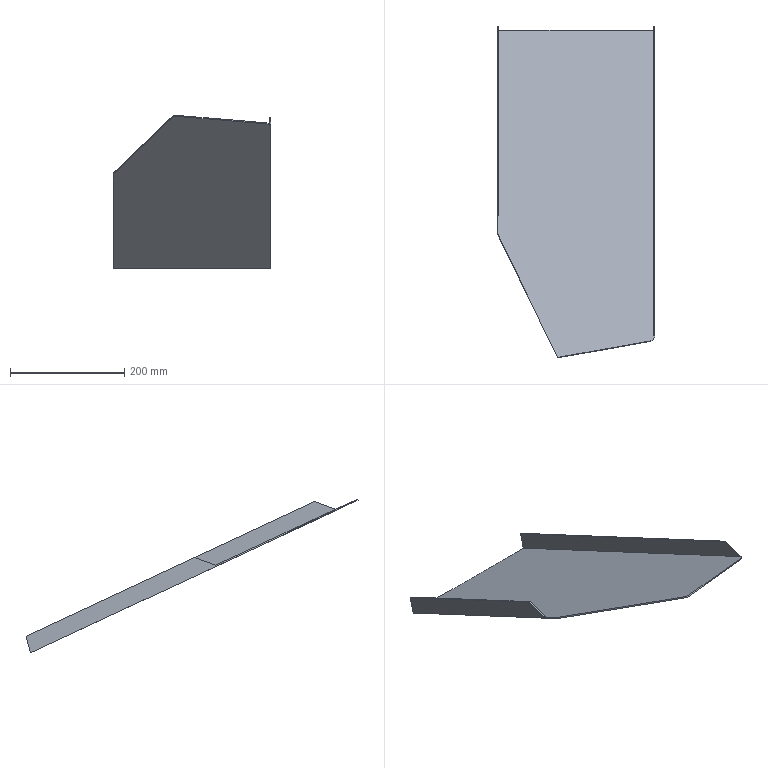Part | NX | features solid 2 | 1 solid | 17 faces | box 276.285 x 582.097 x 269.572 mm | volume 369670 mm3 | plane 16 | spline 1
STEP:
#1=CARTESIAN_POINT('',(829.951,330.323,-255.874));
#2=VERTEX_POINT('',#1);
#3=CARTESIAN_POINT('',(829.951,866.287,-505.798));
#4=VERTEX_POINT('',#3);
#5=CARTESIAN_POINT('',(829.951,540.514,-353.888));
#6=DIRECTION('',(0.,0.9063,-0.4226));
#7=VECTOR('',#6,1000.);
#8=LINE('',#5,#7);
#9=EDGE_CURVE('',#2,#4,#8,.T.);
#10=ORIENTED_EDGE('',*,*,#9,.T.);
#11=CARTESIAN_POINT('',(558.256,866.287,-505.798));
#12=VERTEX_POINT('',#11);
#13=CARTESIAN_POINT('',(831.95,866.287,-505.798));
#14=DIRECTION('',(-1.,0.,0.));
#15=VECTOR('',#14,1000.);
#16=LINE('',#13,#15);
#17=EDGE_CURVE('',#4,#12,#16,.T.);
#18=ORIENTED_EDGE('',*,*,#17,.T.);
#19=CARTESIAN_POINT('',(558.256,540.845,-354.042));
#20=VERTEX_POINT('',#19);
#21=CARTESIAN_POINT('',(558.256,540.514,-353.888));
#22=DIRECTION('',(0.,0.9063,-0.4226));
#23=VECTOR('',#22,1000.);
#24=LINE('',#21,#23);
#25=EDGE_CURVE('',#20,#12,#24,.T.);
#26=ORIENTED_EDGE('',*,*,#25,.F.);
#27=CARTESIAN_POINT('',(556.256,540.845,-354.042));
#28=VERTEX_POINT('',#27);
#29=CARTESIAN_POINT('',(556.256,540.845,-354.042));
#30=DIRECTION('',(-1.,0.,0.));
#31=VECTOR('',#30,1000.);
#32=LINE('',#29,#31);
#33=EDGE_CURVE('',#20,#28,#32,.T.);
#34=ORIENTED_EDGE('',*,*,#33,.T.);
#35=CARTESIAN_POINT('',(555.666,540.845,-354.042));
#36=VERTEX_POINT('',#35);
#37=CARTESIAN_POINT('',(555.666,540.845,-354.042));
#38=DIRECTION('',(1.,0.,0.));
#39=VECTOR('',#38,1000.);
#40=LINE('',#37,#39);
#41=EDGE_CURVE('',#36,#28,#40,.T.);
#42=ORIENTED_EDGE('',*,*,#41,.F.);
#43=CARTESIAN_POINT('',(555.666,510.845,-340.053));
#44=VERTEX_POINT('',#43);
#45=CARTESIAN_POINT('',(555.666,510.845,-340.053));
#46=DIRECTION('',(0.,0.9063,-0.4226));
#47=VECTOR('',#46,1000.);
#48=LINE('',#45,#47);
#49=EDGE_CURVE('',#44,#36,#48,.T.);
#50=ORIENTED_EDGE('',*,*,#49,.F.);
#51=CARTESIAN_POINT('',(556.256,510.845,-340.053));
#52=VERTEX_POINT('',#51);
#53=CARTESIAN_POINT('',(555.666,510.845,-340.053));
#54=DIRECTION('',(1.,0.,0.));
#55=VECTOR('',#54,1000.);
#56=LINE('',#53,#55);
#57=EDGE_CURVE('',#44,#52,#56,.T.);
#58=ORIENTED_EDGE('',*,*,#57,.T.);
#59=CARTESIAN_POINT('',(556.256,509.627,-339.485));
#60=VERTEX_POINT('',#59);
#61=CARTESIAN_POINT('',(556.256,510.845,-340.053));
#62=DIRECTION('',(0.,-0.9063,0.4226));
#63=VECTOR('',#62,1000.);
#64=LINE('',#61,#63);
#65=EDGE_CURVE('',#52,#60,#64,.T.);
#66=ORIENTED_EDGE('',*,*,#65,.T.);
#67=CARTESIAN_POINT('',(661.488,292.393,-238.187));
#68=VERTEX_POINT('',#67);
#69=CARTESIAN_POINT('',(556.256,509.627,-339.485));
#70=DIRECTION('',(0.402,-0.8299,0.387));
#71=VECTOR('',#70,1000.);
#72=LINE('',#69,#71);
#73=EDGE_CURVE('',#60,#68,#72,.T.);
#74=ORIENTED_EDGE('',*,*,#73,.T.);
#75=CARTESIAN_POINT('',(831.951,330.323,-255.874));
#76=VERTEX_POINT('',#75);
#77=CARTESIAN_POINT('',(831.951,330.323,-255.874));
#78=CARTESIAN_POINT('',(831.936,330.109,-255.774));
#79=CARTESIAN_POINT('',(831.91,329.897,-255.675));
#80=CARTESIAN_POINT('',(831.843,329.477,-255.48));
#81=CARTESIAN_POINT('',(831.802,329.269,-255.382));
#82=CARTESIAN_POINT('',(831.703,328.856,-255.19));
#83=CARTESIAN_POINT('',(831.646,328.652,-255.095));
#84=CARTESIAN_POINT('',(831.519,328.246,-254.906));
#85=CARTESIAN_POINT('',(831.448,328.045,-254.812));
#86=CARTESIAN_POINT('',(831.294,327.646,-254.626));
#87=CARTESIAN_POINT('',(831.21,327.448,-254.534));
#88=CARTESIAN_POINT('',(831.074,327.154,-254.396));
#89=CARTESIAN_POINT('',(831.027,327.056,-254.351));
#90=CARTESIAN_POINT('',(830.955,326.91,-254.283));
#91=CARTESIAN_POINT('',(830.93,326.861,-254.26));
#92=CARTESIAN_POINT('',(830.88,326.765,-254.215));
#93=CARTESIAN_POINT('',(830.753,326.524,-254.102));
#94=CARTESIAN_POINT('',(830.619,326.287,-253.992));
#95=CARTESIAN_POINT('',(830.392,325.916,-253.819));
#96=CARTESIAN_POINT('',(830.156,325.55,-253.649));
#97=CARTESIAN_POINT('',(829.771,325.02,-253.401));
#98=CARTESIAN_POINT('',(829.495,324.678,-253.242));
#99=CARTESIAN_POINT('',(829.208,324.342,-253.085));
#100=CARTESIAN_POINT('',(829.06,324.177,-253.008));
#101=CARTESIAN_POINT('',(828.829,323.935,-252.895));
#102=CARTESIAN_POINT('',(828.751,323.855,-252.858));
#103=CARTESIAN_POINT('',(828.592,323.697,-252.784));
#104=CARTESIAN_POINT('',(828.512,323.619,-252.748));
#105=CARTESIAN_POINT('',(828.268,323.389,-252.641));
#106=CARTESIAN_POINT('',(828.101,323.24,-252.572));
#107=CARTESIAN_POINT('',(827.758,322.952,-252.437));
#108=CARTESIAN_POINT('',(827.582,322.813,-252.372));
#109=CARTESIAN_POINT('',(827.222,322.544,-252.247));
#110=CARTESIAN_POINT('',(827.037,322.415,-252.187));
#111=CARTESIAN_POINT('',(826.657,322.167,-252.071));
#112=CARTESIAN_POINT('',(826.462,322.049,-252.016));
#113=CARTESIAN_POINT('',(826.211,321.908,-251.95));
#114=CARTESIAN_POINT('',(826.161,321.881,-251.938));
#115=CARTESIAN_POINT('',(826.059,321.826,-251.912));
#116=CARTESIAN_POINT('',(826.008,321.799,-251.9));
#117=CARTESIAN_POINT('',(825.854,321.72,-251.863));
#118=CARTESIAN_POINT('',(825.75,321.67,-251.839));
#119=CARTESIAN_POINT('',(825.438,321.524,-251.771));
#120=CARTESIAN_POINT('',(825.226,321.435,-251.73));
#121=CARTESIAN_POINT('',(824.797,321.276,-251.655));
#122=CARTESIAN_POINT('',(824.579,321.205,-251.622));
#123=CARTESIAN_POINT('',(824.247,321.113,-251.58));
#124=CARTESIAN_POINT('',(824.135,321.085,-251.567));
#125=CARTESIAN_POINT('',(823.966,321.048,-251.549));
#126=CARTESIAN_POINT('',(823.881,321.03,-251.541));
#127=CARTESIAN_POINT('',(823.795,321.013,-251.533));
#128=CARTESIAN_POINT('',(823.738,321.003,-251.528));
#129=CARTESIAN_POINT('',(823.71,320.998,-251.526));
#130=CARTESIAN_POINT('',(822.765,320.831,-251.448));
#131=CARTESIAN_POINT('',(820.016,320.346,-251.222));
#132=CARTESIAN_POINT('',(809.936,318.569,-250.393));
#133=CARTESIAN_POINT('',(786.111,314.368,-248.434));
#134=CARTESIAN_POINT('',(734.796,305.32,-244.215));
#135=CARTESIAN_POINT('',(690.811,297.564,-240.598));
#136=CARTESIAN_POINT('',(661.488,292.393,-238.187));
#137=B_SPLINE_CURVE_WITH_KNOTS('',3,(#77,#78,#79,#80,#81,#82,#83,#84,#85,#86,#87,#88,#89,#90,#91,#92,#93,#94,#95,#96,#97,#98,#99,#100,#101,#102,#103,#104,#105,#106,#107,#108,#109,#110,#111,#112,#113,#114,#115,#116,#117,#118,#119,#120,#121,#122,#123,#124,#125,#126,#127,#128,#129,#130,#131,#132,#133,#134,#135,#136),.UNSPECIFIED.,.F.,.F.,(4,2,2,2,2,2,2,2,1,2,1,1,2,2,2,2,2,2,2,2,2,2,2,2,2,2,1,2,2,1,1,1,1,4),(0.,0.003906,0.007812,0.01172,0.01562,0.01953,0.02148,0.02246,0.02344,0.02734,0.03125,0.03516,0.03906,0.04297,0.04492,0.04687,0.05078,0.05469,0.05859,0.0625,0.06348,0.06445,0.06641,0.07031,0.07422,0.07617,0.07715,0.07764,0.07812,0.09375,0.125,0.25,0.5,1.),.UNSPECIFIED.);
#138=EDGE_CURVE('',#76,#68,#137,.T.);
#139=ORIENTED_EDGE('',*,*,#138,.F.);
#140=CARTESIAN_POINT('',(831.951,330.323,-255.874));
#141=DIRECTION('',(1.,0.,0.));
#142=VECTOR('',#141,1000.);
#143=LINE('',#140,#142);
#144=EDGE_CURVE('',#76,#2,#143,.F.);
#145=ORIENTED_EDGE('',*,*,#144,.T.);
#146=EDGE_LOOP('',(#10,#18,#26,#34,#42,#50,#58,#66,#74,#139,#145));
#147=FACE_BOUND('',#146,.T.);
#148=CARTESIAN_POINT('',(831.95,540.514,-353.888));
#149=DIRECTION('',(0.,-0.4226,-0.9063));
#150=DIRECTION('',(0.,0.9063,-0.4226));
#151=AXIS2_PLACEMENT_3D('',#148,#149,#150);
#152=PLANE('',#151);
#153=ADVANCED_FACE('',(#147),#152,.F.);
#154=CARTESIAN_POINT('',(831.951,865.761,-507.76));
#155=VERTEX_POINT('',#154);
#156=CARTESIAN_POINT('',(831.951,329.478,-257.687));
#157=VERTEX_POINT('',#156);
#158=CARTESIAN_POINT('',(831.951,510.,-341.866));
#159=DIRECTION('',(0.,-0.9063,0.4226));
#160=VECTOR('',#159,1000.);
#161=LINE('',#158,#160);
#162=EDGE_CURVE('',#155,#157,#161,.T.);
#163=ORIENTED_EDGE('',*,*,#162,.F.);
#164=CARTESIAN_POINT('',(831.951,873.646,-478.335));
#165=VERTEX_POINT('',#164);
#166=CARTESIAN_POINT('',(831.951,883.403,-441.919));
#167=DIRECTION('',(0.,0.2588,0.9659));
#168=VECTOR('',#167,1000.);
#169=LINE('',#166,#168);
#170=EDGE_CURVE('',#155,#165,#169,.T.);
#171=ORIENTED_EDGE('',*,*,#170,.T.);
#172=CARTESIAN_POINT('',(831.951,367.533,-242.331));
#173=VERTEX_POINT('',#172);
#174=CARTESIAN_POINT('',(831.951,1052.679,-561.82));
#175=DIRECTION('',(0.,-0.9063,0.4226));
#176=VECTOR('',#175,1000.);
#177=LINE('',#174,#176);
#178=EDGE_CURVE('',#165,#173,#177,.T.);
#179=ORIENTED_EDGE('',*,*,#178,.T.);
#180=CARTESIAN_POINT('',(831.951,330.323,-255.874));
#181=DIRECTION('',(0.,-0.9397,-0.342));
#182=VECTOR('',#181,1000.);
#183=LINE('',#180,#182);
#184=EDGE_CURVE('',#173,#76,#183,.T.);
#185=ORIENTED_EDGE('',*,*,#184,.T.);
#186=CARTESIAN_POINT('',(831.951,329.478,-257.687));
#187=DIRECTION('',(0.,0.4226,0.9063));
#188=VECTOR('',#187,1000.);
#189=LINE('',#186,#188);
#190=EDGE_CURVE('',#157,#76,#189,.T.);
#191=ORIENTED_EDGE('',*,*,#190,.F.);
#192=EDGE_LOOP('',(#163,#171,#179,#185,#191));
#193=FACE_BOUND('',#192,.T.);
#194=CARTESIAN_POINT('',(831.951,510.,-341.866));
#195=DIRECTION('',(-1.,0.,0.));
#196=DIRECTION('',(0.,0.,1.));
#197=AXIS2_PLACEMENT_3D('',#194,#195,#196);
#198=PLANE('',#197);
#199=ADVANCED_FACE('',(#193),#198,.F.);
#200=ORIENTED_EDGE('',*,*,#138,.T.);
#201=CARTESIAN_POINT('',(661.488,291.548,-240.));
#202=VERTEX_POINT('',#201);
#203=CARTESIAN_POINT('',(661.488,291.548,-240.));
#204=DIRECTION('',(0.,0.4226,0.9063));
#205=VECTOR('',#204,1000.);
#206=LINE('',#203,#205);
#207=EDGE_CURVE('',#202,#68,#206,.T.);
#208=ORIENTED_EDGE('',*,*,#207,.F.);
#209=CARTESIAN_POINT('',(831.951,329.478,-257.687));
#210=CARTESIAN_POINT('',(831.936,329.264,-257.587));
#211=CARTESIAN_POINT('',(831.91,329.052,-257.488));
#212=CARTESIAN_POINT('',(831.843,328.631,-257.292));
#213=CARTESIAN_POINT('',(831.802,328.423,-257.195));
#214=CARTESIAN_POINT('',(831.703,328.011,-257.003));
#215=CARTESIAN_POINT('',(831.646,327.806,-256.907));
#216=CARTESIAN_POINT('',(831.519,327.401,-256.718));
#217=CARTESIAN_POINT('',(831.448,327.2,-256.625));
#218=CARTESIAN_POINT('',(831.294,326.801,-256.439));
#219=CARTESIAN_POINT('',(831.21,326.603,-256.346));
#220=CARTESIAN_POINT('',(831.074,326.309,-256.209));
#221=CARTESIAN_POINT('',(831.027,326.211,-256.163));
#222=CARTESIAN_POINT('',(830.955,326.065,-256.095));
#223=CARTESIAN_POINT('',(830.93,326.016,-256.073));
#224=CARTESIAN_POINT('',(830.88,325.919,-256.028));
#225=CARTESIAN_POINT('',(830.753,325.678,-255.915));
#226=CARTESIAN_POINT('',(830.619,325.442,-255.805));
#227=CARTESIAN_POINT('',(830.392,325.071,-255.632));
#228=CARTESIAN_POINT('',(830.156,324.705,-255.461));
#229=CARTESIAN_POINT('',(829.771,324.175,-255.214));
#230=CARTESIAN_POINT('',(829.495,323.833,-255.055));
#231=CARTESIAN_POINT('',(829.208,323.497,-254.898));
#232=CARTESIAN_POINT('',(829.06,323.332,-254.821));
#233=CARTESIAN_POINT('',(828.829,323.09,-254.708));
#234=CARTESIAN_POINT('',(828.751,323.01,-254.671));
#235=CARTESIAN_POINT('',(828.592,322.852,-254.597));
#236=CARTESIAN_POINT('',(828.512,322.774,-254.561));
#237=CARTESIAN_POINT('',(828.268,322.544,-254.454));
#238=CARTESIAN_POINT('',(828.101,322.395,-254.384));
#239=CARTESIAN_POINT('',(827.758,322.107,-254.25));
#240=CARTESIAN_POINT('',(827.582,321.968,-254.185));
#241=CARTESIAN_POINT('',(827.222,321.699,-254.06));
#242=CARTESIAN_POINT('',(827.037,321.57,-253.999));
#243=CARTESIAN_POINT('',(826.657,321.322,-253.884));
#244=CARTESIAN_POINT('',(826.462,321.204,-253.829));
#245=CARTESIAN_POINT('',(826.211,321.063,-253.763));
#246=CARTESIAN_POINT('',(826.161,321.036,-253.75));
#247=CARTESIAN_POINT('',(826.059,320.981,-253.725));
#248=CARTESIAN_POINT('',(826.008,320.954,-253.712));
#249=CARTESIAN_POINT('',(825.854,320.875,-253.675));
#250=CARTESIAN_POINT('',(825.75,320.824,-253.652));
#251=CARTESIAN_POINT('',(825.438,320.679,-253.584));
#252=CARTESIAN_POINT('',(825.226,320.59,-253.542));
#253=CARTESIAN_POINT('',(824.797,320.43,-253.468));
#254=CARTESIAN_POINT('',(824.579,320.359,-253.435));
#255=CARTESIAN_POINT('',(824.247,320.268,-253.392));
#256=CARTESIAN_POINT('',(824.135,320.24,-253.379));
#257=CARTESIAN_POINT('',(823.966,320.202,-253.362));
#258=CARTESIAN_POINT('',(823.881,320.184,-253.353));
#259=CARTESIAN_POINT('',(823.795,320.168,-253.346));
#260=CARTESIAN_POINT('',(823.738,320.157,-253.341));
#261=CARTESIAN_POINT('',(823.71,320.152,-253.338));
#262=CARTESIAN_POINT('',(822.765,319.986,-253.261));
#263=CARTESIAN_POINT('',(820.016,319.501,-253.035));
#264=CARTESIAN_POINT('',(809.936,317.724,-252.206));
#265=CARTESIAN_POINT('',(786.111,313.523,-250.247));
#266=CARTESIAN_POINT('',(734.796,304.474,-246.028));
#267=CARTESIAN_POINT('',(690.811,296.719,-242.411));
#268=CARTESIAN_POINT('',(661.488,291.548,-240.));
#269=B_SPLINE_CURVE_WITH_KNOTS('',3,(#209,#210,#211,#212,#213,#214,#215,#216,#217,#218,#219,#220,#221,#222,#223,#224,#225,#226,#227,#228,#229,#230,#231,#232,#233,#234,#235,#236,#237,#238,#239,#240,#241,#242,#243,#244,#245,#246,#247,#248,#249,#250,#251,#252,#253,#254,#255,#256,#257,#258,#259,#260,#261,#262,#263,#264,#265,#266,#267,#268),.UNSPECIFIED.,.F.,.F.,(4,2,2,2,2,2,2,2,1,2,1,1,2,2,2,2,2,2,2,2,2,2,2,2,2,2,1,2,2,1,1,1,1,4),(0.,0.003906,0.007812,0.01172,0.01562,0.01953,0.02148,0.02246,0.02344,0.02734,0.03125,0.03516,0.03906,0.04297,0.04492,0.04687,0.05078,0.05469,0.05859,0.0625,0.06348,0.06445,0.06641,0.07031,0.07422,0.07617,0.07715,0.07764,0.07812,0.09375,0.125,0.25,0.5,1.),.UNSPECIFIED.);
#270=EDGE_CURVE('',#157,#202,#269,.T.);
#271=ORIENTED_EDGE('',*,*,#270,.F.);
#272=ORIENTED_EDGE('',*,*,#190,.T.);
#273=EDGE_LOOP('',(#200,#208,#271,#272));
#274=FACE_BOUND('',#273,.T.);
#275=CARTESIAN_POINT('',(831.951,329.478,-257.687));
#276=CARTESIAN_POINT('',(831.951,330.323,-255.874));
#277=CARTESIAN_POINT('',(831.824,327.763,-256.887));
#278=CARTESIAN_POINT('',(831.824,328.609,-255.075));
#279=CARTESIAN_POINT('',(830.805,325.343,-255.759));
#280=CARTESIAN_POINT('',(830.805,326.188,-253.946));
#281=CARTESIAN_POINT('',(828.504,322.631,-254.494));
#282=CARTESIAN_POINT('',(828.504,323.476,-252.681));
#283=CARTESIAN_POINT('',(826.699,321.267,-253.858));
#284=CARTESIAN_POINT('',(826.699,322.112,-252.046));
#285=CARTESIAN_POINT('',(825.025,320.467,-253.485));
#286=CARTESIAN_POINT('',(825.025,321.312,-251.672));
#287=CARTESIAN_POINT('',(823.689,320.127,-253.326));
#288=CARTESIAN_POINT('',(823.689,320.972,-251.514));
#289=CARTESIAN_POINT('',(822.304,319.91,-253.225));
#290=CARTESIAN_POINT('',(822.304,320.755,-251.413));
#291=CARTESIAN_POINT('',(819.56,319.414,-252.994));
#292=CARTESIAN_POINT('',(819.56,320.259,-251.181));
#293=CARTESIAN_POINT('',(815.433,318.696,-252.659));
#294=CARTESIAN_POINT('',(815.433,319.541,-250.846));
#295=CARTESIAN_POINT('',(809.936,317.723,-252.205));
#296=CARTESIAN_POINT('',(809.936,318.568,-250.393));
#297=CARTESIAN_POINT('',(804.438,316.754,-251.754));
#298=CARTESIAN_POINT('',(804.438,317.6,-249.941));
#299=CARTESIAN_POINT('',(798.94,315.785,-251.302));
#300=CARTESIAN_POINT('',(798.94,316.63,-249.489));
#301=CARTESIAN_POINT('',(791.609,314.492,-250.699));
#302=CARTESIAN_POINT('',(791.609,315.337,-248.886));
#303=CARTESIAN_POINT('',(782.446,312.876,-249.945));
#304=CARTESIAN_POINT('',(782.446,313.722,-248.133));
#305=CARTESIAN_POINT('',(767.784,310.291,-248.74));
#306=CARTESIAN_POINT('',(767.784,311.136,-246.927));
#307=CARTESIAN_POINT('',(734.796,304.474,-246.028));
#308=CARTESIAN_POINT('',(734.796,305.32,-244.215));
#309=CARTESIAN_POINT('',(698.142,298.011,-243.014));
#310=CARTESIAN_POINT('',(698.142,298.857,-241.201));
#311=CARTESIAN_POINT('',(668.819,292.841,-240.603));
#312=CARTESIAN_POINT('',(668.819,293.686,-238.79));
#313=CARTESIAN_POINT('',(661.488,291.548,-240.));
#314=CARTESIAN_POINT('',(661.488,292.393,-238.187));
#315=B_SPLINE_SURFACE_WITH_KNOTS('',3,1,((#275,#276),(#277,#278),(#279,#280),(#281,#282),(#283,#284),(#285,#286),(#287,#288),(#289,#290),(#291,#292),(#293,#294),(#295,#296),(#297,#298),(#299,#300),(#301,#302),(#303,#304),(#305,#306),(#307,#308),(#309,#310),(#311,#312),(#313,#314)),.UNSPECIFIED.,.F.,.F.,.F.,(4,1,1,1,1,1,1,1,1,1,1,1,1,1,1,1,1,4),(2,2),(0.,0.03125,0.04688,0.0625,0.07031,0.07812,0.08594,0.09375,0.125,0.1562,0.1875,0.2188,0.25,0.3125,0.375,0.5,0.875,1.),(0.,1.),.UNSPECIFIED.);
#316=ADVANCED_FACE('',(#274),#315,.F.);
#317=ORIENTED_EDGE('',*,*,#73,.F.);
#318=CARTESIAN_POINT('',(556.256,508.781,-341.297));
#319=VERTEX_POINT('',#318);
#320=CARTESIAN_POINT('',(556.256,508.781,-341.297));
#321=DIRECTION('',(0.,0.4226,0.9063));
#322=VECTOR('',#321,1000.);
#323=LINE('',#320,#322);
#324=EDGE_CURVE('',#319,#60,#323,.T.);
#325=ORIENTED_EDGE('',*,*,#324,.F.);
#326=CARTESIAN_POINT('',(556.256,508.781,-341.297));
#327=DIRECTION('',(0.402,-0.8299,0.387));
#328=VECTOR('',#327,1000.);
#329=LINE('',#326,#328);
#330=EDGE_CURVE('',#319,#202,#329,.T.);
#331=ORIENTED_EDGE('',*,*,#330,.T.);
#332=ORIENTED_EDGE('',*,*,#207,.T.);
#333=EDGE_LOOP('',(#317,#325,#331,#332));
#334=FACE_BOUND('',#333,.T.);
#335=CARTESIAN_POINT('',(556.256,508.781,-341.297));
#336=DIRECTION('',(-0.9156,-0.3643,0.1699));
#337=DIRECTION('',(0.3697,-0.9291,0.));
#338=AXIS2_PLACEMENT_3D('',#335,#336,#337);
#339=PLANE('',#338);
#340=ADVANCED_FACE('',(#334),#339,.T.);
#341=ORIENTED_EDGE('',*,*,#65,.F.);
#342=CARTESIAN_POINT('',(556.256,510.,-341.866));
#343=VERTEX_POINT('',#342);
#344=CARTESIAN_POINT('',(556.256,510.,-341.866));
#345=DIRECTION('',(0.,0.4226,0.9063));
#346=VECTOR('',#345,1000.);
#347=LINE('',#344,#346);
#348=EDGE_CURVE('',#343,#52,#347,.T.);
#349=ORIENTED_EDGE('',*,*,#348,.F.);
#350=CARTESIAN_POINT('',(556.256,510.,-341.866));
#351=DIRECTION('',(0.,-0.9063,0.4226));
#352=VECTOR('',#351,1000.);
#353=LINE('',#350,#352);
#354=EDGE_CURVE('',#343,#319,#353,.T.);
#355=ORIENTED_EDGE('',*,*,#354,.T.);
#356=ORIENTED_EDGE('',*,*,#324,.T.);
#357=EDGE_LOOP('',(#341,#349,#355,#356));
#358=FACE_BOUND('',#357,.T.);
#359=CARTESIAN_POINT('',(556.256,510.,-341.866));
#360=DIRECTION('',(-1.,0.,0.));
#361=DIRECTION('',(0.,0.,1.));
#362=AXIS2_PLACEMENT_3D('',#359,#360,#361);
#363=PLANE('',#362);
#364=ADVANCED_FACE('',(#358),#363,.T.);
#365=ORIENTED_EDGE('',*,*,#57,.F.);
#366=CARTESIAN_POINT('',(555.666,510.,-341.866));
#367=VERTEX_POINT('',#366);
#368=CARTESIAN_POINT('',(555.666,510.,-341.866));
#369=DIRECTION('',(0.,0.4226,0.9063));
#370=VECTOR('',#369,1000.);
#371=LINE('',#368,#370);
#372=EDGE_CURVE('',#367,#44,#371,.T.);
#373=ORIENTED_EDGE('',*,*,#372,.F.);
#374=CARTESIAN_POINT('',(555.666,510.,-341.866));
#375=DIRECTION('',(1.,0.,0.));
#376=VECTOR('',#375,1000.);
#377=LINE('',#374,#376);
#378=EDGE_CURVE('',#367,#343,#377,.T.);
#379=ORIENTED_EDGE('',*,*,#378,.T.);
#380=ORIENTED_EDGE('',*,*,#348,.T.);
#381=EDGE_LOOP('',(#365,#373,#379,#380));
#382=FACE_BOUND('',#381,.T.);
#383=CARTESIAN_POINT('',(555.666,510.,-341.866));
#384=DIRECTION('',(0.,-0.9063,0.4226));
#385=DIRECTION('',(0.,-0.4226,-0.9063));
#386=AXIS2_PLACEMENT_3D('',#383,#384,#385);
#387=PLANE('',#386);
#388=ADVANCED_FACE('',(#382),#387,.T.);
#389=ORIENTED_EDGE('',*,*,#49,.T.);
#390=CARTESIAN_POINT('',(555.666,540.,-355.855));
#391=VERTEX_POINT('',#390);
#392=CARTESIAN_POINT('',(555.666,540.,-355.855));
#393=DIRECTION('',(0.,0.4226,0.9063));
#394=VECTOR('',#393,1000.);
#395=LINE('',#392,#394);
#396=EDGE_CURVE('',#391,#36,#395,.T.);
#397=ORIENTED_EDGE('',*,*,#396,.F.);
#398=CARTESIAN_POINT('',(555.666,510.,-341.866));
#399=DIRECTION('',(0.,0.9063,-0.4226));
#400=VECTOR('',#399,1000.);
#401=LINE('',#398,#400);
#402=EDGE_CURVE('',#367,#391,#401,.T.);
#403=ORIENTED_EDGE('',*,*,#402,.F.);
#404=ORIENTED_EDGE('',*,*,#372,.T.);
#405=EDGE_LOOP('',(#389,#397,#403,#404));
#406=FACE_BOUND('',#405,.T.);
#407=CARTESIAN_POINT('',(555.666,510.,-341.866));
#408=DIRECTION('',(1.,0.,0.));
#409=DIRECTION('',(0.,0.,-1.));
#410=AXIS2_PLACEMENT_3D('',#407,#408,#409);
#411=PLANE('',#410);
#412=ADVANCED_FACE('',(#406),#411,.F.);
#413=ORIENTED_EDGE('',*,*,#41,.T.);
#414=CARTESIAN_POINT('',(556.256,540.,-355.855));
#415=VERTEX_POINT('',#414);
#416=CARTESIAN_POINT('',(556.256,540.,-355.855));
#417=DIRECTION('',(0.,0.4226,0.9063));
#418=VECTOR('',#417,1000.);
#419=LINE('',#416,#418);
#420=EDGE_CURVE('',#415,#28,#419,.T.);
#421=ORIENTED_EDGE('',*,*,#420,.F.);
#422=CARTESIAN_POINT('',(555.666,540.,-355.855));
#423=DIRECTION('',(1.,0.,0.));
#424=VECTOR('',#423,1000.);
#425=LINE('',#422,#424);
#426=EDGE_CURVE('',#391,#415,#425,.T.);
#427=ORIENTED_EDGE('',*,*,#426,.F.);
#428=ORIENTED_EDGE('',*,*,#396,.T.);
#429=EDGE_LOOP('',(#413,#421,#427,#428));
#430=FACE_BOUND('',#429,.T.);
#431=CARTESIAN_POINT('',(555.666,540.,-355.855));
#432=DIRECTION('',(0.,-0.9063,0.4226));
#433=DIRECTION('',(0.,-0.4226,-0.9063));
#434=AXIS2_PLACEMENT_3D('',#431,#432,#433);
#435=PLANE('',#434);
#436=ADVANCED_FACE('',(#430),#435,.F.);
#437=CARTESIAN_POINT('',(556.256,865.761,-507.76));
#438=VERTEX_POINT('',#437);
#439=CARTESIAN_POINT('',(556.256,873.646,-478.335));
#440=VERTEX_POINT('',#439);
#441=CARTESIAN_POINT('',(556.256,862.576,-519.649));
#442=DIRECTION('',(0.,0.2588,0.9659));
#443=VECTOR('',#442,1000.);
#444=LINE('',#441,#443);
#445=EDGE_CURVE('',#438,#440,#444,.T.);
#446=ORIENTED_EDGE('',*,*,#445,.F.);
#447=CARTESIAN_POINT('',(556.256,930.,-537.715));
#448=DIRECTION('',(0.,-0.9063,0.4226));
#449=VECTOR('',#448,1000.);
#450=LINE('',#447,#449);
#451=EDGE_CURVE('',#438,#415,#450,.T.);
#452=ORIENTED_EDGE('',*,*,#451,.T.);
#453=ORIENTED_EDGE('',*,*,#420,.T.);
#454=CARTESIAN_POINT('',(556.256,578.055,-340.499));
#455=VERTEX_POINT('',#454);
#456=CARTESIAN_POINT('',(556.256,906.093,-221.103));
#457=DIRECTION('',(0.,0.9397,0.342));
#458=VECTOR('',#457,1000.);
#459=LINE('',#456,#458);
#460=EDGE_CURVE('',#28,#455,#459,.T.);
#461=ORIENTED_EDGE('',*,*,#460,.T.);
#462=CARTESIAN_POINT('',(556.256,1052.679,-561.82));
#463=DIRECTION('',(0.,-0.9063,0.4226));
#464=VECTOR('',#463,1000.);
#465=LINE('',#462,#464);
#466=EDGE_CURVE('',#440,#455,#465,.T.);
#467=ORIENTED_EDGE('',*,*,#466,.F.);
#468=EDGE_LOOP('',(#446,#452,#453,#461,#467));
#469=FACE_BOUND('',#468,.T.);
#470=CARTESIAN_POINT('',(556.256,930.,-537.715));
#471=DIRECTION('',(-1.,0.,0.));
#472=DIRECTION('',(0.,-1.,0.));
#473=AXIS2_PLACEMENT_3D('',#470,#471,#472);
#474=PLANE('',#473);
#475=ADVANCED_FACE('',(#469),#474,.T.);
#476=CARTESIAN_POINT('',(831.95,865.761,-507.76));
#477=DIRECTION('',(-1.,0.,0.));
#478=VECTOR('',#477,1000.);
#479=LINE('',#476,#478);
#480=EDGE_CURVE('',#155,#438,#479,.T.);
#481=ORIENTED_EDGE('',*,*,#480,.F.);
#482=ORIENTED_EDGE('',*,*,#162,.T.);
#483=ORIENTED_EDGE('',*,*,#270,.T.);
#484=ORIENTED_EDGE('',*,*,#330,.F.);
#485=ORIENTED_EDGE('',*,*,#354,.F.);
#486=ORIENTED_EDGE('',*,*,#378,.F.);
#487=ORIENTED_EDGE('',*,*,#402,.T.);
#488=ORIENTED_EDGE('',*,*,#426,.T.);
#489=ORIENTED_EDGE('',*,*,#451,.F.);
#490=EDGE_LOOP('',(#481,#482,#483,#484,#485,#486,#487,#488,#489));
#491=FACE_BOUND('',#490,.T.);
#492=CARTESIAN_POINT('',(831.95,539.669,-355.701));
#493=DIRECTION('',(0.,-0.4226,-0.9063));
#494=DIRECTION('',(0.,0.9063,-0.4226));
#495=AXIS2_PLACEMENT_3D('',#492,#493,#494);
#496=PLANE('',#495);
#497=ADVANCED_FACE('',(#491),#496,.T.);
#498=ORIENTED_EDGE('',*,*,#25,.T.);
#499=CARTESIAN_POINT('',(558.256,873.646,-478.335));
#500=VERTEX_POINT('',#499);
#501=CARTESIAN_POINT('',(558.256,857.121,-540.006));
#502=DIRECTION('',(0.,0.2588,0.9659));
#503=VECTOR('',#502,1000.);
#504=LINE('',#501,#503);
#505=EDGE_CURVE('',#12,#500,#504,.T.);
#506=ORIENTED_EDGE('',*,*,#505,.T.);
#507=CARTESIAN_POINT('',(558.256,578.055,-340.499));
#508=VERTEX_POINT('',#507);
#509=CARTESIAN_POINT('',(558.256,1052.679,-561.82));
#510=DIRECTION('',(0.,-0.9063,0.4226));
#511=VECTOR('',#510,1000.);
#512=LINE('',#509,#511);
#513=EDGE_CURVE('',#500,#508,#512,.T.);
#514=ORIENTED_EDGE('',*,*,#513,.T.);
#515=CARTESIAN_POINT('',(558.256,578.055,-340.499));
#516=DIRECTION('',(0.,-0.9397,-0.342));
#517=VECTOR('',#516,1000.);
#518=LINE('',#515,#517);
#519=EDGE_CURVE('',#508,#20,#518,.T.);
#520=ORIENTED_EDGE('',*,*,#519,.T.);
#521=EDGE_LOOP('',(#498,#506,#514,#520));
#522=FACE_BOUND('',#521,.T.);
#523=CARTESIAN_POINT('',(558.256,1040.,-589.009));
#524=DIRECTION('',(-1.,0.,0.));
#525=DIRECTION('',(0.,-1.,0.));
#526=AXIS2_PLACEMENT_3D('',#523,#524,#525);
#527=PLANE('',#526);
#528=ADVANCED_FACE('',(#522),#527,.F.);
#529=CARTESIAN_POINT('',(556.256,873.646,-478.335));
#530=DIRECTION('',(-1.,0.,0.));
#531=VECTOR('',#530,1000.);
#532=LINE('',#529,#531);
#533=EDGE_CURVE('',#440,#500,#532,.F.);
#534=ORIENTED_EDGE('',*,*,#533,.F.);
#535=ORIENTED_EDGE('',*,*,#466,.T.);
#536=CARTESIAN_POINT('',(556.256,578.055,-340.499));
#537=DIRECTION('',(-1.,0.,0.));
#538=VECTOR('',#537,1000.);
#539=LINE('',#536,#538);
#540=EDGE_CURVE('',#455,#508,#539,.F.);
#541=ORIENTED_EDGE('',*,*,#540,.T.);
#542=ORIENTED_EDGE('',*,*,#513,.F.);
#543=EDGE_LOOP('',(#534,#535,#541,#542));
#544=FACE_BOUND('',#543,.T.);
#545=CARTESIAN_POINT('',(556.256,1052.679,-561.82));
#546=DIRECTION('',(0.,-0.4226,-0.9063));
#547=DIRECTION('',(0.,-0.9063,0.4226));
#548=AXIS2_PLACEMENT_3D('',#545,#546,#547);
#549=PLANE('',#548);
#550=ADVANCED_FACE('',(#544),#549,.F.);
#551=ORIENTED_EDGE('',*,*,#460,.F.);
#552=ORIENTED_EDGE('',*,*,#33,.F.);
#553=ORIENTED_EDGE('',*,*,#519,.F.);
#554=ORIENTED_EDGE('',*,*,#540,.F.);
#555=EDGE_LOOP('',(#551,#552,#553,#554));
#556=FACE_BOUND('',#555,.T.);
#557=CARTESIAN_POINT('',(556.256,578.055,-340.499));
#558=DIRECTION('',(0.,-0.342,0.9397));
#559=DIRECTION('',(0.,-0.9397,-0.342));
#560=AXIS2_PLACEMENT_3D('',#557,#558,#559);
#561=PLANE('',#560);
#562=ADVANCED_FACE('',(#556),#561,.T.);
#563=CARTESIAN_POINT('',(829.951,873.646,-478.335));
#564=VERTEX_POINT('',#563);
#565=CARTESIAN_POINT('',(829.951,857.121,-540.006));
#566=DIRECTION('',(0.,0.2588,0.9659));
#567=VECTOR('',#566,1000.);
#568=LINE('',#565,#567);
#569=EDGE_CURVE('',#4,#564,#568,.T.);
#570=ORIENTED_EDGE('',*,*,#569,.F.);
#571=ORIENTED_EDGE('',*,*,#9,.F.);
#572=CARTESIAN_POINT('',(829.951,367.533,-242.331));
#573=VERTEX_POINT('',#572);
#574=CARTESIAN_POINT('',(829.951,849.916,-66.758));
#575=DIRECTION('',(0.,0.9397,0.342));
#576=VECTOR('',#575,1000.);
#577=LINE('',#574,#576);
#578=EDGE_CURVE('',#2,#573,#577,.T.);
#579=ORIENTED_EDGE('',*,*,#578,.T.);
#580=CARTESIAN_POINT('',(829.951,1052.679,-561.82));
#581=DIRECTION('',(0.,-0.9063,0.4226));
#582=VECTOR('',#581,1000.);
#583=LINE('',#580,#582);
#584=EDGE_CURVE('',#564,#573,#583,.T.);
#585=ORIENTED_EDGE('',*,*,#584,.F.);
#586=EDGE_LOOP('',(#570,#571,#579,#585));
#587=FACE_BOUND('',#586,.T.);
#588=CARTESIAN_POINT('',(829.951,1040.,-589.009));
#589=DIRECTION('',(-1.,0.,0.));
#590=DIRECTION('',(0.,0.,1.));
#591=AXIS2_PLACEMENT_3D('',#588,#589,#590);
#592=PLANE('',#591);
#593=ADVANCED_FACE('',(#587),#592,.T.);
#594=ORIENTED_EDGE('',*,*,#178,.F.);
#595=CARTESIAN_POINT('',(831.951,873.646,-478.335));
#596=DIRECTION('',(-1.,0.,0.));
#597=VECTOR('',#596,1000.);
#598=LINE('',#595,#597);
#599=EDGE_CURVE('',#165,#564,#598,.T.);
#600=ORIENTED_EDGE('',*,*,#599,.T.);
#601=ORIENTED_EDGE('',*,*,#584,.T.);
#602=CARTESIAN_POINT('',(831.951,367.533,-242.331));
#603=DIRECTION('',(1.,0.,0.));
#604=VECTOR('',#603,1000.);
#605=LINE('',#602,#604);
#606=EDGE_CURVE('',#573,#173,#605,.T.);
#607=ORIENTED_EDGE('',*,*,#606,.T.);
#608=EDGE_LOOP('',(#594,#600,#601,#607));
#609=FACE_BOUND('',#608,.T.);
#610=CARTESIAN_POINT('',(831.951,1052.679,-561.82));
#611=DIRECTION('',(0.,-0.4226,-0.9063));
#612=DIRECTION('',(0.,-0.9063,0.4226));
#613=AXIS2_PLACEMENT_3D('',#610,#611,#612);
#614=PLANE('',#613);
#615=ADVANCED_FACE('',(#609),#614,.F.);
#616=ORIENTED_EDGE('',*,*,#184,.F.);
#617=ORIENTED_EDGE('',*,*,#606,.F.);
#618=ORIENTED_EDGE('',*,*,#578,.F.);
#619=ORIENTED_EDGE('',*,*,#144,.F.);
#620=EDGE_LOOP('',(#616,#617,#618,#619));
#621=FACE_BOUND('',#620,.T.);
#622=CARTESIAN_POINT('',(831.951,330.323,-255.874));
#623=DIRECTION('',(0.,-0.342,0.9397));
#624=DIRECTION('',(0.,-0.9397,-0.342));
#625=AXIS2_PLACEMENT_3D('',#622,#623,#624);
#626=PLANE('',#625);
#627=ADVANCED_FACE('',(#621),#626,.T.);
#628=ORIENTED_EDGE('',*,*,#445,.T.);
#629=ORIENTED_EDGE('',*,*,#533,.T.);
#630=ORIENTED_EDGE('',*,*,#505,.F.);
#631=ORIENTED_EDGE('',*,*,#17,.F.);
#632=ORIENTED_EDGE('',*,*,#569,.T.);
#633=ORIENTED_EDGE('',*,*,#599,.F.);
#634=ORIENTED_EDGE('',*,*,#170,.F.);
#635=ORIENTED_EDGE('',*,*,#480,.T.);
#636=EDGE_LOOP('',(#628,#629,#630,#631,#632,#633,#634,#635));
#637=FACE_BOUND('',#636,.T.);
#638=CARTESIAN_POINT('',(546.256,864.593,-512.118));
#639=DIRECTION('',(0.,-0.9659,0.2588));
#640=DIRECTION('',(0.,-0.2588,-0.9659));
#641=AXIS2_PLACEMENT_3D('',#638,#639,#640);
#642=PLANE('',#641);
#643=ADVANCED_FACE('',(#637),#642,.F.);
#644=CLOSED_SHELL('',(#153,#199,#316,#340,#364,#388,#412,#436,#475,#497,#528,#550,#562,#593,#615,#627,#643));
#645=MANIFOLD_SOLID_BREP('',#644);
#646=(LENGTH_UNIT()NAMED_UNIT(*)SI_UNIT(.MILLI.,.METRE.));
#647=UNCERTAINTY_MEASURE_WITH_UNIT(LENGTH_MEASURE(0.0508),#646,'','');
#648=(NAMED_UNIT(*)PLANE_ANGLE_UNIT()SI_UNIT($,.RADIAN.));
#649=(NAMED_UNIT(*)SI_UNIT($,.STERADIAN.)SOLID_ANGLE_UNIT());
#650=(GEOMETRIC_REPRESENTATION_CONTEXT(3)GLOBAL_UNCERTAINTY_ASSIGNED_CONTEXT((#647))GLOBAL_UNIT_ASSIGNED_CONTEXT((#646,#648,#649))REPRESENTATION_CONTEXT('',''));
#651=ADVANCED_BREP_SHAPE_REPRESENTATION('',(#645),#650);